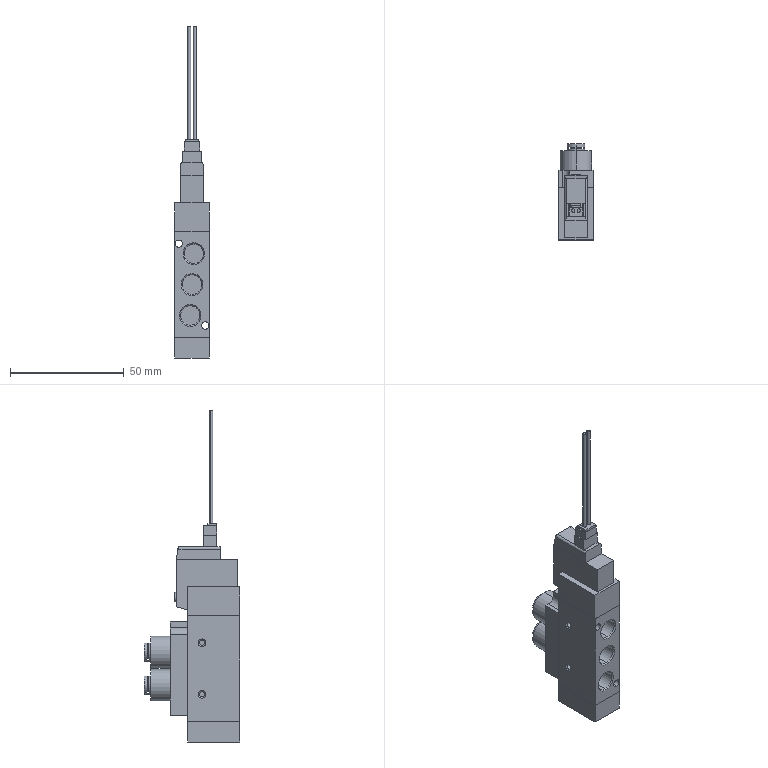Part | SolidWorks | features Boss 25, Cut 6, RevCut 5, Revolution 2, Extrusion 1, ICE 1 | 1 solid | 153 faces | box 15.02 x 42.2 x 146.05 mm | volume 33782 mm3 | plane 99 | cylinder 44 | cone 10 | commonest cylinder face diameters 7.9 x8 8.57 x6 1.5 x4 2.46 x4 3.2 x4 4 x4